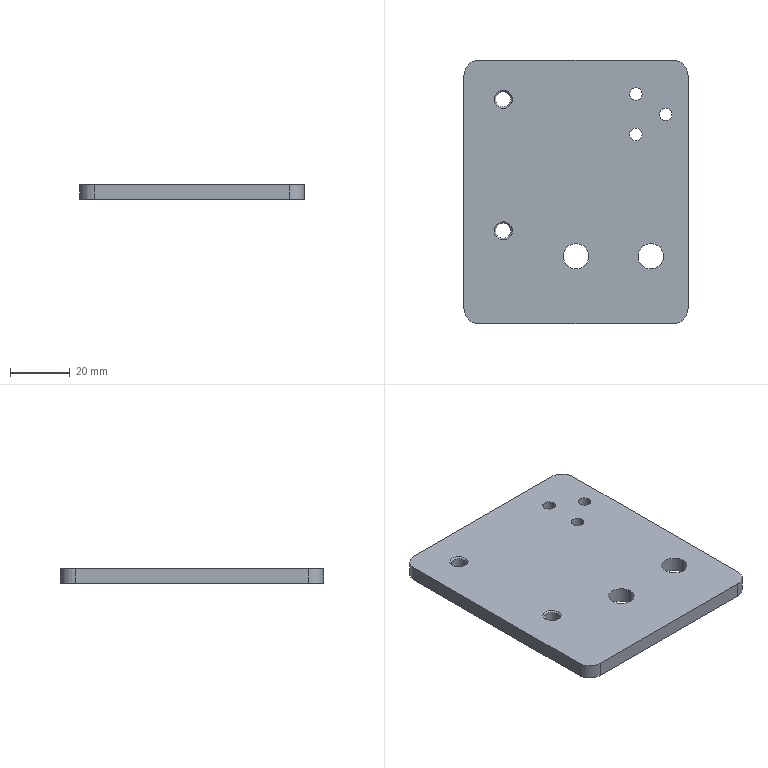Part | STEP file | 1 solid | 28 faces | box 75 x 88 x 5 mm | volume 31916 mm3 | cylinder 18 | plane 6 | cone 4 | commonest cylinder face diameters 4.2 x6 5 x4 8.5 x4 10 x4